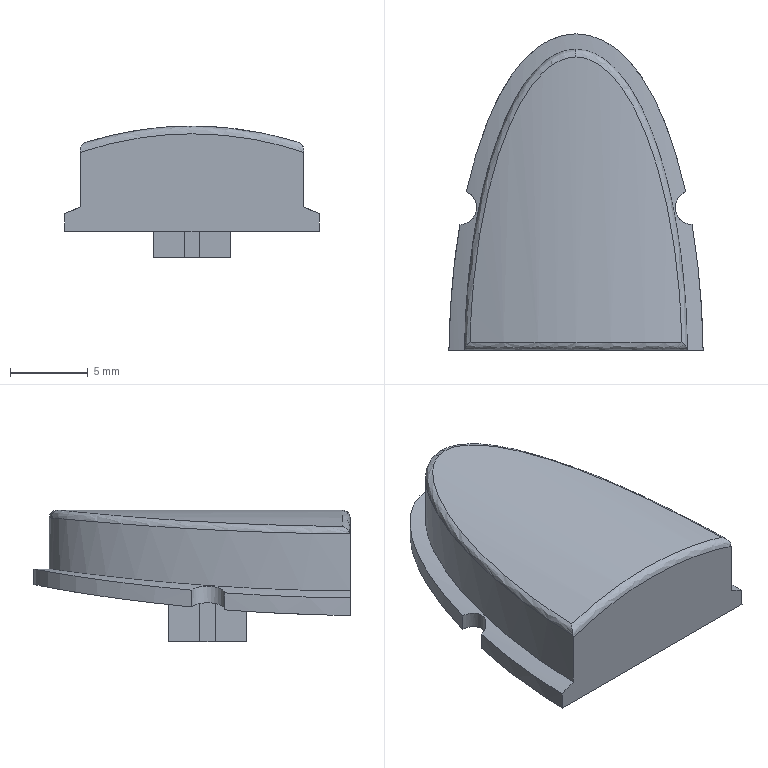Part | STEP file | 1 solid | 33 faces | box 16.389 x 20.4 x 8.5 mm | volume 856.443 mm3 | plane 16 | spline 11 | cylinder 6 | commonest cylinder face diameters 2.2 x2 36 x1 38 x1 41.6 x1 45.6 x1